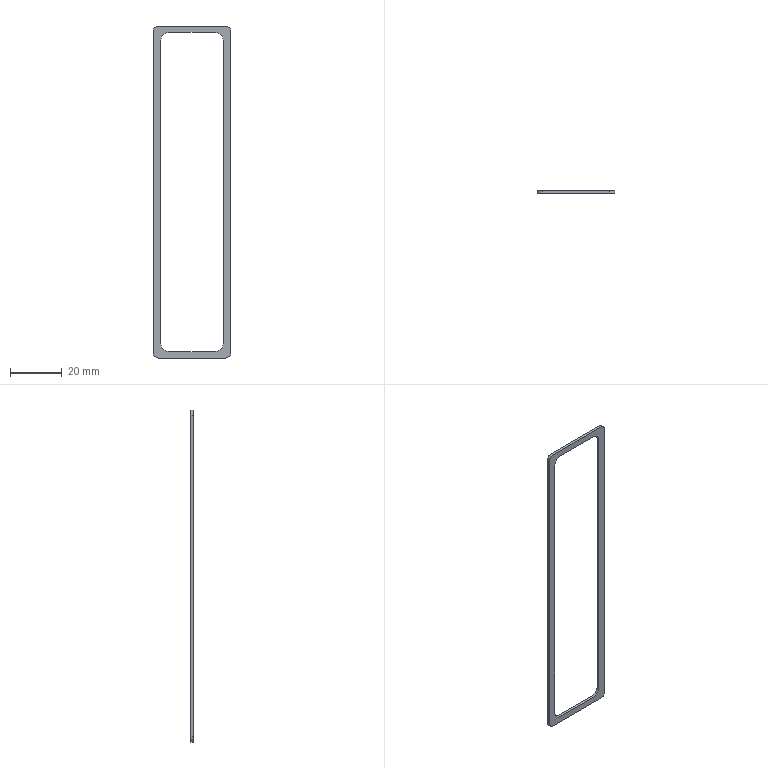Part | STEP file | _X2_751F4E45_X0_MS731-1_X2_8F_6 | 1 solid | 18 faces | box 30 x 1 x 128 mm | volume 892.292 mm3 | plane 10 | cylinder 8 | commonest cylinder face diameters 4 x4 6 x4
STEP:
#1=CARTESIAN_POINT('',(0.,0.,0.));
#2=DIRECTION('',(0.,0.,1.));
#3=DIRECTION('',(1.,0.,0.));
#4=AXIS2_PLACEMENT_3D('',#1,#2,#3);
#5=CARTESIAN_POINT('',(0.5,21.681,-127.));
#6=VERTEX_POINT('',#5);
#7=CARTESIAN_POINT('',(0.5,21.681,-3.));
#8=VERTEX_POINT('',#7);
#9=CARTESIAN_POINT('',(0.5,21.681,-127.));
#10=DIRECTION('',(0.,0.,1.));
#11=VECTOR('',#10,1.);
#12=LINE('',#9,#11);
#13=CARTESIAN_POINT('',(15.5,21.681,-65.));
#14=DIRECTION('',(0.,1.,0.));
#15=DIRECTION('',(-1.,0.,0.));
#16=AXIS2_PLACEMENT_3D('',#13,#14,#15);
#17=PLANE('',#16);
#18=CARTESIAN_POINT('',(15.,-62.));
#19=DIRECTION('',(0.,1.));
#20=VECTOR('',#19,1.);
#21=LINE('',#18,#20);
#22=(GEOMETRIC_REPRESENTATION_CONTEXT(2)PARAMETRIC_REPRESENTATION_CONTEXT()REPRESENTATION_CONTEXT('',''));
#23=DEFINITIONAL_REPRESENTATION('',(#21),#22);
#24=PCURVE('',#17,#23);
#25=CARTESIAN_POINT('',(0.5,21.681,-129.));
#26=DIRECTION('',(-1.,0.,0.));
#27=DIRECTION('',(0.,0.,-1.));
#28=AXIS2_PLACEMENT_3D('',#25,#26,#27);
#29=PLANE('',#28);
#30=CARTESIAN_POINT('',(-2.,0.));
#31=DIRECTION('',(-1.,0.));
#32=VECTOR('',#31,1.);
#33=LINE('',#30,#32);
#34=(GEOMETRIC_REPRESENTATION_CONTEXT(2)PARAMETRIC_REPRESENTATION_CONTEXT()REPRESENTATION_CONTEXT('',''));
#35=DEFINITIONAL_REPRESENTATION('',(#33),#34);
#36=PCURVE('',#29,#35);
#37=SURFACE_CURVE('',#12,(#24,#36),.PCURVE_S1.);
#38=EDGE_CURVE('',#6,#8,#37,.T.);
#39=ORIENTED_EDGE('',*,*,#38,.T.);
#40=CARTESIAN_POINT('',(2.5,21.681,-1.));
#41=VERTEX_POINT('',#40);
#42=CARTESIAN_POINT('',(2.5,21.681,-3.));
#43=DIRECTION('',(0.,-1.,0.));
#44=DIRECTION('',(0.,0.,1.));
#45=AXIS2_PLACEMENT_3D('',#42,#43,#44);
#46=CIRCLE('',#45,2.);
#47=CARTESIAN_POINT('',(13.,64.));
#48=CARTESIAN_POINT('',(16.464,64.));
#49=CARTESIAN_POINT('',(14.732,61.));
#50=CARTESIAN_POINT('',(13.,58.));
#51=CARTESIAN_POINT('',(11.268,61.));
#52=CARTESIAN_POINT('',(9.536,64.));
#53=CARTESIAN_POINT('',(13.,64.));
#54=(BOUNDED_CURVE()B_SPLINE_CURVE(2,(#47,#48,#49,#50,#51,#52,#53),.UNSPECIFIED.,.T.,.F.)B_SPLINE_CURVE_WITH_KNOTS((1,2,2,2,2,1),(-2.094,0.,2.094,4.189,6.283,8.378),.UNSPECIFIED.)CURVE()GEOMETRIC_REPRESENTATION_ITEM()RATIONAL_B_SPLINE_CURVE((1.,0.5,1.,0.5,1.,0.5,1.))REPRESENTATION_ITEM(''));
#55=(GEOMETRIC_REPRESENTATION_CONTEXT(2)PARAMETRIC_REPRESENTATION_CONTEXT()REPRESENTATION_CONTEXT('',''));
#56=DEFINITIONAL_REPRESENTATION('',(#54),#55);
#57=PCURVE('',#17,#56);
#58=CARTESIAN_POINT('',(2.5,22.908,-3.));
#59=DIRECTION('',(0.,-1.,0.));
#60=DIRECTION('',(0.,0.,-1.));
#61=AXIS2_PLACEMENT_3D('',#58,#59,#60);
#62=CYLINDRICAL_SURFACE('',#61,2.);
#63=CARTESIAN_POINT('',(3.142,1.226));
#64=DIRECTION('',(1.,0.));
#65=VECTOR('',#64,1.);
#66=LINE('',#63,#65);
#67=(GEOMETRIC_REPRESENTATION_CONTEXT(2)PARAMETRIC_REPRESENTATION_CONTEXT()REPRESENTATION_CONTEXT('',''));
#68=DEFINITIONAL_REPRESENTATION('',(#66),#67);
#69=PCURVE('',#62,#68);
#70=SURFACE_CURVE('',#46,(#57,#69),.PCURVE_S1.);
#71=EDGE_CURVE('',#41,#8,#70,.T.);
#72=ORIENTED_EDGE('',*,*,#71,.F.);
#73=CARTESIAN_POINT('',(28.5,21.681,-1.));
#74=VERTEX_POINT('',#73);
#75=CARTESIAN_POINT('',(2.5,21.681,-1.));
#76=DIRECTION('',(1.,0.,0.));
#77=VECTOR('',#76,1.);
#78=LINE('',#75,#77);
#79=CARTESIAN_POINT('',(13.,64.));
#80=DIRECTION('',(-1.,0.));
#81=VECTOR('',#80,1.);
#82=LINE('',#79,#81);
#83=(GEOMETRIC_REPRESENTATION_CONTEXT(2)PARAMETRIC_REPRESENTATION_CONTEXT()REPRESENTATION_CONTEXT('',''));
#84=DEFINITIONAL_REPRESENTATION('',(#82),#83);
#85=PCURVE('',#17,#84);
#86=CARTESIAN_POINT('',(0.5,21.681,-1.));
#87=DIRECTION('',(0.,0.,1.));
#88=DIRECTION('',(-1.,0.,0.));
#89=AXIS2_PLACEMENT_3D('',#86,#87,#88);
#90=PLANE('',#89);
#91=CARTESIAN_POINT('',(-2.,0.));
#92=DIRECTION('',(-1.,0.));
#93=VECTOR('',#92,1.);
#94=LINE('',#91,#93);
#95=(GEOMETRIC_REPRESENTATION_CONTEXT(2)PARAMETRIC_REPRESENTATION_CONTEXT()REPRESENTATION_CONTEXT('',''));
#96=DEFINITIONAL_REPRESENTATION('',(#94),#95);
#97=PCURVE('',#90,#96);
#98=SURFACE_CURVE('',#78,(#85,#97),.PCURVE_S1.);
#99=EDGE_CURVE('',#41,#74,#98,.T.);
#100=ORIENTED_EDGE('',*,*,#99,.T.);
#101=CARTESIAN_POINT('',(30.5,21.681,-3.));
#102=VERTEX_POINT('',#101);
#103=CARTESIAN_POINT('',(28.5,21.681,-3.));
#104=DIRECTION('',(0.,-1.,0.));
#105=DIRECTION('',(1.,0.,0.));
#106=AXIS2_PLACEMENT_3D('',#103,#104,#105);
#107=CIRCLE('',#106,2.);
#108=CARTESIAN_POINT('',(-15.,62.));
#109=CARTESIAN_POINT('',(-15.,65.464));
#110=CARTESIAN_POINT('',(-12.,63.732));
#111=CARTESIAN_POINT('',(-9.,62.));
#112=CARTESIAN_POINT('',(-12.,60.268));
#113=CARTESIAN_POINT('',(-15.,58.536));
#114=CARTESIAN_POINT('',(-15.,62.));
#115=(BOUNDED_CURVE()B_SPLINE_CURVE(2,(#108,#109,#110,#111,#112,#113,#114),.UNSPECIFIED.,.T.,.F.)B_SPLINE_CURVE_WITH_KNOTS((1,2,2,2,2,1),(-2.094,0.,2.094,4.189,6.283,8.378),.UNSPECIFIED.)CURVE()GEOMETRIC_REPRESENTATION_ITEM()RATIONAL_B_SPLINE_CURVE((1.,0.5,1.,0.5,1.,0.5,1.))REPRESENTATION_ITEM(''));
#116=(GEOMETRIC_REPRESENTATION_CONTEXT(2)PARAMETRIC_REPRESENTATION_CONTEXT()REPRESENTATION_CONTEXT('',''));
#117=DEFINITIONAL_REPRESENTATION('',(#115),#116);
#118=PCURVE('',#17,#117);
#119=CARTESIAN_POINT('',(28.5,22.908,-3.));
#120=DIRECTION('',(0.,-1.,0.));
#121=DIRECTION('',(-1.,0.,0.));
#122=AXIS2_PLACEMENT_3D('',#119,#120,#121);
#123=CYLINDRICAL_SURFACE('',#122,2.);
#124=CARTESIAN_POINT('',(3.142,1.226));
#125=DIRECTION('',(1.,0.));
#126=VECTOR('',#125,1.);
#127=LINE('',#124,#126);
#128=(GEOMETRIC_REPRESENTATION_CONTEXT(2)PARAMETRIC_REPRESENTATION_CONTEXT()REPRESENTATION_CONTEXT('',''));
#129=DEFINITIONAL_REPRESENTATION('',(#127),#128);
#130=PCURVE('',#123,#129);
#131=SURFACE_CURVE('',#107,(#118,#130),.PCURVE_S1.);
#132=EDGE_CURVE('',#102,#74,#131,.T.);
#133=ORIENTED_EDGE('',*,*,#132,.F.);
#134=CARTESIAN_POINT('',(30.5,21.681,-127.));
#135=VERTEX_POINT('',#134);
#136=CARTESIAN_POINT('',(30.5,21.681,-3.));
#137=DIRECTION('',(0.,0.,-1.));
#138=VECTOR('',#137,1.);
#139=LINE('',#136,#138);
#140=CARTESIAN_POINT('',(-15.,62.));
#141=DIRECTION('',(0.,-1.));
#142=VECTOR('',#141,1.);
#143=LINE('',#140,#142);
#144=(GEOMETRIC_REPRESENTATION_CONTEXT(2)PARAMETRIC_REPRESENTATION_CONTEXT()REPRESENTATION_CONTEXT('',''));
#145=DEFINITIONAL_REPRESENTATION('',(#143),#144);
#146=PCURVE('',#17,#145);
#147=CARTESIAN_POINT('',(30.5,21.681,-1.));
#148=DIRECTION('',(1.,0.,0.));
#149=DIRECTION('',(0.,0.,1.));
#150=AXIS2_PLACEMENT_3D('',#147,#148,#149);
#151=PLANE('',#150);
#152=CARTESIAN_POINT('',(-2.,0.));
#153=DIRECTION('',(-1.,0.));
#154=VECTOR('',#153,1.);
#155=LINE('',#152,#154);
#156=(GEOMETRIC_REPRESENTATION_CONTEXT(2)PARAMETRIC_REPRESENTATION_CONTEXT()REPRESENTATION_CONTEXT('',''));
#157=DEFINITIONAL_REPRESENTATION('',(#155),#156);
#158=PCURVE('',#151,#157);
#159=SURFACE_CURVE('',#139,(#146,#158),.PCURVE_S1.);
#160=EDGE_CURVE('',#102,#135,#159,.T.);
#161=ORIENTED_EDGE('',*,*,#160,.T.);
#162=CARTESIAN_POINT('',(28.5,21.681,-129.));
#163=VERTEX_POINT('',#162);
#164=CARTESIAN_POINT('',(28.5,21.681,-127.));
#165=DIRECTION('',(0.,-1.,0.));
#166=DIRECTION('',(0.,0.,-1.));
#167=AXIS2_PLACEMENT_3D('',#164,#165,#166);
#168=CIRCLE('',#167,2.);
#169=CARTESIAN_POINT('',(-13.,-64.));
#170=CARTESIAN_POINT('',(-16.464,-64.));
#171=CARTESIAN_POINT('',(-14.732,-61.));
#172=CARTESIAN_POINT('',(-13.,-58.));
#173=CARTESIAN_POINT('',(-11.268,-61.));
#174=CARTESIAN_POINT('',(-9.536,-64.));
#175=CARTESIAN_POINT('',(-13.,-64.));
#176=(BOUNDED_CURVE()B_SPLINE_CURVE(2,(#169,#170,#171,#172,#173,#174,#175),.UNSPECIFIED.,.T.,.F.)B_SPLINE_CURVE_WITH_KNOTS((1,2,2,2,2,1),(-2.094,0.,2.094,4.189,6.283,8.378),.UNSPECIFIED.)CURVE()GEOMETRIC_REPRESENTATION_ITEM()RATIONAL_B_SPLINE_CURVE((1.,0.5,1.,0.5,1.,0.5,1.))REPRESENTATION_ITEM(''));
#177=(GEOMETRIC_REPRESENTATION_CONTEXT(2)PARAMETRIC_REPRESENTATION_CONTEXT()REPRESENTATION_CONTEXT('',''));
#178=DEFINITIONAL_REPRESENTATION('',(#176),#177);
#179=PCURVE('',#17,#178);
#180=CARTESIAN_POINT('',(28.5,22.908,-127.));
#181=DIRECTION('',(0.,-1.,0.));
#182=DIRECTION('',(0.,0.,1.));
#183=AXIS2_PLACEMENT_3D('',#180,#181,#182);
#184=CYLINDRICAL_SURFACE('',#183,2.);
#185=CARTESIAN_POINT('',(3.142,1.226));
#186=DIRECTION('',(1.,0.));
#187=VECTOR('',#186,1.);
#188=LINE('',#185,#187);
#189=(GEOMETRIC_REPRESENTATION_CONTEXT(2)PARAMETRIC_REPRESENTATION_CONTEXT()REPRESENTATION_CONTEXT('',''));
#190=DEFINITIONAL_REPRESENTATION('',(#188),#189);
#191=PCURVE('',#184,#190);
#192=SURFACE_CURVE('',#168,(#179,#191),.PCURVE_S1.);
#193=EDGE_CURVE('',#163,#135,#192,.T.);
#194=ORIENTED_EDGE('',*,*,#193,.F.);
#195=CARTESIAN_POINT('',(2.5,21.681,-129.));
#196=VERTEX_POINT('',#195);
#197=CARTESIAN_POINT('',(28.5,21.681,-129.));
#198=DIRECTION('',(-1.,0.,0.));
#199=VECTOR('',#198,1.);
#200=LINE('',#197,#199);
#201=CARTESIAN_POINT('',(-13.,-64.));
#202=DIRECTION('',(1.,0.));
#203=VECTOR('',#202,1.);
#204=LINE('',#201,#203);
#205=(GEOMETRIC_REPRESENTATION_CONTEXT(2)PARAMETRIC_REPRESENTATION_CONTEXT()REPRESENTATION_CONTEXT('',''));
#206=DEFINITIONAL_REPRESENTATION('',(#204),#205);
#207=PCURVE('',#17,#206);
#208=CARTESIAN_POINT('',(30.5,21.681,-129.));
#209=DIRECTION('',(0.,0.,-1.));
#210=DIRECTION('',(1.,0.,0.));
#211=AXIS2_PLACEMENT_3D('',#208,#209,#210);
#212=PLANE('',#211);
#213=CARTESIAN_POINT('',(-2.,0.));
#214=DIRECTION('',(-1.,0.));
#215=VECTOR('',#214,1.);
#216=LINE('',#213,#215);
#217=(GEOMETRIC_REPRESENTATION_CONTEXT(2)PARAMETRIC_REPRESENTATION_CONTEXT()REPRESENTATION_CONTEXT('',''));
#218=DEFINITIONAL_REPRESENTATION('',(#216),#217);
#219=PCURVE('',#212,#218);
#220=SURFACE_CURVE('',#200,(#207,#219),.PCURVE_S1.);
#221=EDGE_CURVE('',#163,#196,#220,.T.);
#222=ORIENTED_EDGE('',*,*,#221,.T.);
#223=CARTESIAN_POINT('',(2.5,21.681,-127.));
#224=DIRECTION('',(0.,-1.,0.));
#225=DIRECTION('',(-1.,0.,0.));
#226=AXIS2_PLACEMENT_3D('',#223,#224,#225);
#227=CIRCLE('',#226,2.);
#228=CARTESIAN_POINT('',(15.,-62.));
#229=CARTESIAN_POINT('',(15.,-65.464));
#230=CARTESIAN_POINT('',(12.,-63.732));
#231=CARTESIAN_POINT('',(9.,-62.));
#232=CARTESIAN_POINT('',(12.,-60.268));
#233=CARTESIAN_POINT('',(15.,-58.536));
#234=CARTESIAN_POINT('',(15.,-62.));
#235=(BOUNDED_CURVE()B_SPLINE_CURVE(2,(#228,#229,#230,#231,#232,#233,#234),.UNSPECIFIED.,.T.,.F.)B_SPLINE_CURVE_WITH_KNOTS((1,2,2,2,2,1),(-2.094,0.,2.094,4.189,6.283,8.378),.UNSPECIFIED.)CURVE()GEOMETRIC_REPRESENTATION_ITEM()RATIONAL_B_SPLINE_CURVE((1.,0.5,1.,0.5,1.,0.5,1.))REPRESENTATION_ITEM(''));
#236=(GEOMETRIC_REPRESENTATION_CONTEXT(2)PARAMETRIC_REPRESENTATION_CONTEXT()REPRESENTATION_CONTEXT('',''));
#237=DEFINITIONAL_REPRESENTATION('',(#235),#236);
#238=PCURVE('',#17,#237);
#239=CARTESIAN_POINT('',(2.5,22.908,-127.));
#240=DIRECTION('',(0.,-1.,0.));
#241=DIRECTION('',(1.,0.,0.));
#242=AXIS2_PLACEMENT_3D('',#239,#240,#241);
#243=CYLINDRICAL_SURFACE('',#242,2.);
#244=CARTESIAN_POINT('',(3.142,1.226));
#245=DIRECTION('',(1.,0.));
#246=VECTOR('',#245,1.);
#247=LINE('',#244,#246);
#248=(GEOMETRIC_REPRESENTATION_CONTEXT(2)PARAMETRIC_REPRESENTATION_CONTEXT()REPRESENTATION_CONTEXT('',''));
#249=DEFINITIONAL_REPRESENTATION('',(#247),#248);
#250=PCURVE('',#243,#249);
#251=SURFACE_CURVE('',#227,(#238,#250),.PCURVE_S1.);
#252=EDGE_CURVE('',#6,#196,#251,.T.);
#253=ORIENTED_EDGE('',*,*,#252,.F.);
#254=EDGE_LOOP('',(#39,#72,#100,#133,#161,#194,#222,#253));
#255=FACE_BOUND('',#254,.F.);
#256=CARTESIAN_POINT('',(6.5,21.681,-126.5));
#257=VERTEX_POINT('',#256);
#258=CARTESIAN_POINT('',(3.5,21.681,-123.5));
#259=VERTEX_POINT('',#258);
#260=CARTESIAN_POINT('',(6.5,21.681,-123.5));
#261=DIRECTION('',(0.,1.,0.));
#262=DIRECTION('',(0.,0.,-1.));
#263=AXIS2_PLACEMENT_3D('',#260,#261,#262);
#264=CIRCLE('',#263,3.);
#265=CARTESIAN_POINT('',(9.,-58.5));
#266=DIRECTION('',(0.,-1.));
#267=AXIS2_PLACEMENT_2D('',#265,#266);
#268=CIRCLE('',#267,3.);
#269=(GEOMETRIC_REPRESENTATION_CONTEXT(2)PARAMETRIC_REPRESENTATION_CONTEXT()REPRESENTATION_CONTEXT('',''));
#270=DEFINITIONAL_REPRESENTATION('',(#268),#269);
#271=PCURVE('',#17,#270);
#272=CARTESIAN_POINT('',(6.5,21.488,-123.5));
#273=DIRECTION('',(0.,1.,0.));
#274=DIRECTION('',(0.,0.,1.));
#275=AXIS2_PLACEMENT_3D('',#272,#273,#274);
#276=CYLINDRICAL_SURFACE('',#275,3.);
#277=CARTESIAN_POINT('',(3.142,0.1933));
#278=DIRECTION('',(1.,0.));
#279=VECTOR('',#278,1.);
#280=LINE('',#277,#279);
#281=(GEOMETRIC_REPRESENTATION_CONTEXT(2)PARAMETRIC_REPRESENTATION_CONTEXT()REPRESENTATION_CONTEXT('',''));
#282=DEFINITIONAL_REPRESENTATION('',(#280),#281);
#283=PCURVE('',#276,#282);
#284=SURFACE_CURVE('',#264,(#271,#283),.PCURVE_S1.);
#285=EDGE_CURVE('',#257,#259,#284,.T.);
#286=ORIENTED_EDGE('',*,*,#285,.F.);
#287=CARTESIAN_POINT('',(24.5,21.681,-126.5));
#288=VERTEX_POINT('',#287);
#289=CARTESIAN_POINT('',(6.5,21.681,-126.5));
#290=DIRECTION('',(1.,0.,0.));
#291=VECTOR('',#290,1.);
#292=LINE('',#289,#291);
#293=CARTESIAN_POINT('',(9.,-61.5));
#294=DIRECTION('',(-1.,0.));
#295=VECTOR('',#294,1.);
#296=LINE('',#293,#295);
#297=(GEOMETRIC_REPRESENTATION_CONTEXT(2)PARAMETRIC_REPRESENTATION_CONTEXT()REPRESENTATION_CONTEXT('',''));
#298=DEFINITIONAL_REPRESENTATION('',(#296),#297);
#299=PCURVE('',#17,#298);
#300=CARTESIAN_POINT('',(3.5,21.681,-126.5));
#301=DIRECTION('',(0.,0.,1.));
#302=DIRECTION('',(-1.,0.,0.));
#303=AXIS2_PLACEMENT_3D('',#300,#301,#302);
#304=PLANE('',#303);
#305=CARTESIAN_POINT('',(-3.,0.));
#306=DIRECTION('',(-1.,0.));
#307=VECTOR('',#306,1.);
#308=LINE('',#305,#307);
#309=(GEOMETRIC_REPRESENTATION_CONTEXT(2)PARAMETRIC_REPRESENTATION_CONTEXT()REPRESENTATION_CONTEXT('',''));
#310=DEFINITIONAL_REPRESENTATION('',(#308),#309);
#311=PCURVE('',#304,#310);
#312=SURFACE_CURVE('',#292,(#299,#311),.PCURVE_S1.);
#313=EDGE_CURVE('',#257,#288,#312,.T.);
#314=ORIENTED_EDGE('',*,*,#313,.T.);
#315=CARTESIAN_POINT('',(27.5,21.681,-123.5));
#316=VERTEX_POINT('',#315);
#317=CARTESIAN_POINT('',(24.5,21.681,-123.5));
#318=DIRECTION('',(0.,1.,0.));
#319=DIRECTION('',(1.,0.,0.));
#320=AXIS2_PLACEMENT_3D('',#317,#318,#319);
#321=CIRCLE('',#320,3.);
#322=CARTESIAN_POINT('',(-9.,-58.5));
#323=DIRECTION('',(-1.,0.));
#324=AXIS2_PLACEMENT_2D('',#322,#323);
#325=CIRCLE('',#324,3.);
#326=(GEOMETRIC_REPRESENTATION_CONTEXT(2)PARAMETRIC_REPRESENTATION_CONTEXT()REPRESENTATION_CONTEXT('',''));
#327=DEFINITIONAL_REPRESENTATION('',(#325),#326);
#328=PCURVE('',#17,#327);
#329=CARTESIAN_POINT('',(24.5,21.488,-123.5));
#330=DIRECTION('',(0.,1.,0.));
#331=DIRECTION('',(-1.,0.,0.));
#332=AXIS2_PLACEMENT_3D('',#329,#330,#331);
#333=CYLINDRICAL_SURFACE('',#332,3.);
#334=CARTESIAN_POINT('',(3.142,0.1933));
#335=DIRECTION('',(1.,0.));
#336=VECTOR('',#335,1.);
#337=LINE('',#334,#336);
#338=(GEOMETRIC_REPRESENTATION_CONTEXT(2)PARAMETRIC_REPRESENTATION_CONTEXT()REPRESENTATION_CONTEXT('',''));
#339=DEFINITIONAL_REPRESENTATION('',(#337),#338);
#340=PCURVE('',#333,#339);
#341=SURFACE_CURVE('',#321,(#328,#340),.PCURVE_S1.);
#342=EDGE_CURVE('',#316,#288,#341,.T.);
#343=ORIENTED_EDGE('',*,*,#342,.F.);
#344=CARTESIAN_POINT('',(27.5,21.681,-6.5));
#345=VERTEX_POINT('',#344);
#346=CARTESIAN_POINT('',(27.5,21.681,-123.5));
#347=DIRECTION('',(0.,0.,1.));
#348=VECTOR('',#347,1.);
#349=LINE('',#346,#348);
#350=CARTESIAN_POINT('',(-12.,-58.5));
#351=DIRECTION('',(0.,1.));
#352=VECTOR('',#351,1.);
#353=LINE('',#350,#352);
#354=(GEOMETRIC_REPRESENTATION_CONTEXT(2)PARAMETRIC_REPRESENTATION_CONTEXT()REPRESENTATION_CONTEXT('',''));
#355=DEFINITIONAL_REPRESENTATION('',(#353),#354);
#356=PCURVE('',#17,#355);
#357=CARTESIAN_POINT('',(27.5,21.681,-126.5));
#358=DIRECTION('',(-1.,0.,0.));
#359=DIRECTION('',(0.,0.,-1.));
#360=AXIS2_PLACEMENT_3D('',#357,#358,#359);
#361=PLANE('',#360);
#362=CARTESIAN_POINT('',(-3.,0.));
#363=DIRECTION('',(-1.,0.));
#364=VECTOR('',#363,1.);
#365=LINE('',#362,#364);
#366=(GEOMETRIC_REPRESENTATION_CONTEXT(2)PARAMETRIC_REPRESENTATION_CONTEXT()REPRESENTATION_CONTEXT('',''));
#367=DEFINITIONAL_REPRESENTATION('',(#365),#366);
#368=PCURVE('',#361,#367);
#369=SURFACE_CURVE('',#349,(#356,#368),.PCURVE_S1.);
#370=EDGE_CURVE('',#316,#345,#369,.T.);
#371=ORIENTED_EDGE('',*,*,#370,.T.);
#372=CARTESIAN_POINT('',(24.5,21.681,-3.5));
#373=VERTEX_POINT('',#372);
#374=CARTESIAN_POINT('',(24.5,21.681,-6.5));
#375=DIRECTION('',(0.,1.,0.));
#376=DIRECTION('',(0.,0.,1.));
#377=AXIS2_PLACEMENT_3D('',#374,#375,#376);
#378=CIRCLE('',#377,3.);
#379=CARTESIAN_POINT('',(-9.,58.5));
#380=DIRECTION('',(0.,1.));
#381=AXIS2_PLACEMENT_2D('',#379,#380);
#382=CIRCLE('',#381,3.);
#383=(GEOMETRIC_REPRESENTATION_CONTEXT(2)PARAMETRIC_REPRESENTATION_CONTEXT()REPRESENTATION_CONTEXT('',''));
#384=DEFINITIONAL_REPRESENTATION('',(#382),#383);
#385=PCURVE('',#17,#384);
#386=CARTESIAN_POINT('',(24.5,21.488,-6.5));
#387=DIRECTION('',(0.,1.,0.));
#388=DIRECTION('',(0.,0.,-1.));
#389=AXIS2_PLACEMENT_3D('',#386,#387,#388);
#390=CYLINDRICAL_SURFACE('',#389,3.);
#391=CARTESIAN_POINT('',(3.142,0.1933));
#392=DIRECTION('',(1.,0.));
#393=VECTOR('',#392,1.);
#394=LINE('',#391,#393);
#395=(GEOMETRIC_REPRESENTATION_CONTEXT(2)PARAMETRIC_REPRESENTATION_CONTEXT()REPRESENTATION_CONTEXT('',''));
#396=DEFINITIONAL_REPRESENTATION('',(#394),#395);
#397=PCURVE('',#390,#396);
#398=SURFACE_CURVE('',#378,(#385,#397),.PCURVE_S1.);
#399=EDGE_CURVE('',#373,#345,#398,.T.);
#400=ORIENTED_EDGE('',*,*,#399,.F.);
#401=CARTESIAN_POINT('',(6.5,21.681,-3.5));
#402=VERTEX_POINT('',#401);
#403=CARTESIAN_POINT('',(24.5,21.681,-3.5));
#404=DIRECTION('',(-1.,0.,0.));
#405=VECTOR('',#404,1.);
#406=LINE('',#403,#405);
#407=CARTESIAN_POINT('',(-9.,61.5));
#408=DIRECTION('',(1.,0.));
#409=VECTOR('',#408,1.);
#410=LINE('',#407,#409);
#411=(GEOMETRIC_REPRESENTATION_CONTEXT(2)PARAMETRIC_REPRESENTATION_CONTEXT()REPRESENTATION_CONTEXT('',''));
#412=DEFINITIONAL_REPRESENTATION('',(#410),#411);
#413=PCURVE('',#17,#412);
#414=CARTESIAN_POINT('',(27.5,21.681,-3.5));
#415=DIRECTION('',(0.,0.,-1.));
#416=DIRECTION('',(1.,0.,0.));
#417=AXIS2_PLACEMENT_3D('',#414,#415,#416);
#418=PLANE('',#417);
#419=CARTESIAN_POINT('',(-3.,0.));
#420=DIRECTION('',(-1.,0.));
#421=VECTOR('',#420,1.);
#422=LINE('',#419,#421);
#423=(GEOMETRIC_REPRESENTATION_CONTEXT(2)PARAMETRIC_REPRESENTATION_CONTEXT()REPRESENTATION_CONTEXT('',''));
#424=DEFINITIONAL_REPRESENTATION('',(#422),#423);
#425=PCURVE('',#418,#424);
#426=SURFACE_CURVE('',#406,(#413,#425),.PCURVE_S1.);
#427=EDGE_CURVE('',#373,#402,#426,.T.);
#428=ORIENTED_EDGE('',*,*,#427,.T.);
#429=CARTESIAN_POINT('',(3.5,21.681,-6.5));
#430=VERTEX_POINT('',#429);
#431=CARTESIAN_POINT('',(6.5,21.681,-6.5));
#432=DIRECTION('',(0.,1.,0.));
#433=DIRECTION('',(-1.,0.,0.));
#434=AXIS2_PLACEMENT_3D('',#431,#432,#433);
#435=CIRCLE('',#434,3.);
#436=CARTESIAN_POINT('',(9.,58.5));
#437=DIRECTION('',(1.,0.));
#438=AXIS2_PLACEMENT_2D('',#436,#437);
#439=CIRCLE('',#438,3.);
#440=(GEOMETRIC_REPRESENTATION_CONTEXT(2)PARAMETRIC_REPRESENTATION_CONTEXT()REPRESENTATION_CONTEXT('',''));
#441=DEFINITIONAL_REPRESENTATION('',(#439),#440);
#442=PCURVE('',#17,#441);
#443=CARTESIAN_POINT('',(6.5,21.488,-6.5));
#444=DIRECTION('',(0.,1.,0.));
#445=DIRECTION('',(1.,0.,0.));
#446=AXIS2_PLACEMENT_3D('',#443,#444,#445);
#447=CYLINDRICAL_SURFACE('',#446,3.);
#448=CARTESIAN_POINT('',(3.142,0.1933));
#449=DIRECTION('',(1.,0.));
#450=VECTOR('',#449,1.);
#451=LINE('',#448,#450);
#452=(GEOMETRIC_REPRESENTATION_CONTEXT(2)PARAMETRIC_REPRESENTATION_CONTEXT()REPRESENTATION_CONTEXT('',''));
#453=DEFINITIONAL_REPRESENTATION('',(#451),#452);
#454=PCURVE('',#447,#453);
#455=SURFACE_CURVE('',#435,(#442,#454),.PCURVE_S1.);
#456=EDGE_CURVE('',#430,#402,#455,.T.);
#457=ORIENTED_EDGE('',*,*,#456,.F.);
#458=CARTESIAN_POINT('',(3.5,21.681,-6.5));
#459=DIRECTION('',(0.,0.,-1.));
#460=VECTOR('',#459,1.);
#461=LINE('',#458,#460);
#462=CARTESIAN_POINT('',(12.,58.5));
#463=DIRECTION('',(0.,-1.));
#464=VECTOR('',#463,1.);
#465=LINE('',#462,#464);
#466=(GEOMETRIC_REPRESENTATION_CONTEXT(2)PARAMETRIC_REPRESENTATION_CONTEXT()REPRESENTATION_CONTEXT('',''));
#467=DEFINITIONAL_REPRESENTATION('',(#465),#466);
#468=PCURVE('',#17,#467);
#469=CARTESIAN_POINT('',(3.5,21.681,-3.5));
#470=DIRECTION('',(1.,0.,0.));
#471=DIRECTION('',(0.,0.,1.));
#472=AXIS2_PLACEMENT_3D('',#469,#470,#471);
#473=PLANE('',#472);
#474=CARTESIAN_POINT('',(-3.,0.));
#475=DIRECTION('',(-1.,0.));
#476=VECTOR('',#475,1.);
#477=LINE('',#474,#476);
#478=(GEOMETRIC_REPRESENTATION_CONTEXT(2)PARAMETRIC_REPRESENTATION_CONTEXT()REPRESENTATION_CONTEXT('',''));
#479=DEFINITIONAL_REPRESENTATION('',(#477),#478);
#480=PCURVE('',#473,#479);
#481=SURFACE_CURVE('',#461,(#468,#480),.PCURVE_S1.);
#482=EDGE_CURVE('',#430,#259,#481,.T.);
#483=ORIENTED_EDGE('',*,*,#482,.T.);
#484=EDGE_LOOP('',(#286,#314,#343,#371,#400,#428,#457,#483));
#485=FACE_BOUND('',#484,.F.);
#486=ADVANCED_FACE('',(#255,#485),#17,.F.);
#487=CARTESIAN_POINT('',(0.5,22.681,-127.));
#488=VERTEX_POINT('',#487);
#489=CARTESIAN_POINT('',(0.5,22.681,-3.));
#490=VERTEX_POINT('',#489);
#491=CARTESIAN_POINT('',(0.5,22.681,-127.));
#492=DIRECTION('',(0.,0.,1.));
#493=VECTOR('',#492,1.);
#494=LINE('',#491,#493);
#495=CARTESIAN_POINT('',(-2.,-1.));
#496=DIRECTION('',(-1.,0.));
#497=VECTOR('',#496,1.);
#498=LINE('',#495,#497);
#499=(GEOMETRIC_REPRESENTATION_CONTEXT(2)PARAMETRIC_REPRESENTATION_CONTEXT()REPRESENTATION_CONTEXT('',''));
#500=DEFINITIONAL_REPRESENTATION('',(#498),#499);
#501=PCURVE('',#29,#500);
#502=CARTESIAN_POINT('',(15.5,22.681,-65.));
#503=DIRECTION('',(0.,1.,0.));
#504=DIRECTION('',(-1.,0.,0.));
#505=AXIS2_PLACEMENT_3D('',#502,#503,#504);
#506=PLANE('',#505);
#507=CARTESIAN_POINT('',(15.,-62.));
#508=DIRECTION('',(0.,1.));
#509=VECTOR('',#508,1.);
#510=LINE('',#507,#509);
#511=(GEOMETRIC_REPRESENTATION_CONTEXT(2)PARAMETRIC_REPRESENTATION_CONTEXT()REPRESENTATION_CONTEXT('',''));
#512=DEFINITIONAL_REPRESENTATION('',(#510),#511);
#513=PCURVE('',#506,#512);
#514=SURFACE_CURVE('',#494,(#501,#513),.PCURVE_S1.);
#515=EDGE_CURVE('',#488,#490,#514,.T.);
#516=ORIENTED_EDGE('',*,*,#515,.T.);
#517=CARTESIAN_POINT('',(0.5,22.681,-3.));
#518=DIRECTION('',(0.,-1.,0.));
#519=VECTOR('',#518,1.);
#520=LINE('',#517,#519);
#521=CARTESIAN_POINT('',(-126.,-1.));
#522=DIRECTION('',(0.,1.));
#523=VECTOR('',#522,1.);
#524=LINE('',#521,#523);
#525=(GEOMETRIC_REPRESENTATION_CONTEXT(2)PARAMETRIC_REPRESENTATION_CONTEXT()REPRESENTATION_CONTEXT('',''));
#526=DEFINITIONAL_REPRESENTATION('',(#524),#525);
#527=PCURVE('',#29,#526);
#528=CARTESIAN_POINT('',(4.712,0.2263));
#529=DIRECTION('',(0.,1.));
#530=VECTOR('',#529,1.);
#531=LINE('',#528,#530);
#532=(GEOMETRIC_REPRESENTATION_CONTEXT(2)PARAMETRIC_REPRESENTATION_CONTEXT()REPRESENTATION_CONTEXT('',''));
#533=DEFINITIONAL_REPRESENTATION('',(#531),#532);
#534=PCURVE('',#62,#533);
#535=SURFACE_CURVE('',#520,(#527,#534),.PCURVE_S1.);
#536=EDGE_CURVE('',#490,#8,#535,.T.);
#537=ORIENTED_EDGE('',*,*,#536,.T.);
#538=ORIENTED_EDGE('',*,*,#38,.F.);
#539=CARTESIAN_POINT('',(0.5,21.681,-127.));
#540=DIRECTION('',(0.,1.,0.));
#541=VECTOR('',#540,1.);
#542=LINE('',#539,#541);
#543=CARTESIAN_POINT('',(-2.,0.));
#544=DIRECTION('',(0.,-1.));
#545=VECTOR('',#544,1.);
#546=LINE('',#543,#545);
#547=(GEOMETRIC_REPRESENTATION_CONTEXT(2)PARAMETRIC_REPRESENTATION_CONTEXT()REPRESENTATION_CONTEXT('',''));
#548=DEFINITIONAL_REPRESENTATION('',(#546),#547);
#549=PCURVE('',#29,#548);
#550=CARTESIAN_POINT('',(3.142,1.226));
#551=DIRECTION('',(0.,-1.));
#552=VECTOR('',#551,1.);
#553=LINE('',#550,#552);
#554=(GEOMETRIC_REPRESENTATION_CONTEXT(2)PARAMETRIC_REPRESENTATION_CONTEXT()REPRESENTATION_CONTEXT('',''));
#555=DEFINITIONAL_REPRESENTATION('',(#553),#554);
#556=PCURVE('',#243,#555);
#557=SURFACE_CURVE('',#542,(#549,#556),.PCURVE_S1.);
#558=EDGE_CURVE('',#6,#488,#557,.T.);
#559=ORIENTED_EDGE('',*,*,#558,.T.);
#560=EDGE_LOOP('',(#516,#537,#538,#559));
#561=FACE_BOUND('',#560,.F.);
#562=ADVANCED_FACE('',(#561),#29,.T.);
#563=CARTESIAN_POINT('',(2.5,22.681,-1.));
#564=VERTEX_POINT('',#563);
#565=CARTESIAN_POINT('',(28.5,22.681,-1.));
#566=VERTEX_POINT('',#565);
#567=CARTESIAN_POINT('',(2.5,22.681,-1.));
#568=DIRECTION('',(1.,0.,0.));
#569=VECTOR('',#568,1.);
#570=LINE('',#567,#569);
#571=CARTESIAN_POINT('',(13.,64.));
#572=DIRECTION('',(-1.,0.));
#573=VECTOR('',#572,1.);
#574=LINE('',#571,#573);
#575=(GEOMETRIC_REPRESENTATION_CONTEXT(2)PARAMETRIC_REPRESENTATION_CONTEXT()REPRESENTATION_CONTEXT('',''));
#576=DEFINITIONAL_REPRESENTATION('',(#574),#575);
#577=PCURVE('',#506,#576);
#578=CARTESIAN_POINT('',(-2.,-1.));
#579=DIRECTION('',(-1.,0.));
#580=VECTOR('',#579,1.);
#581=LINE('',#578,#580);
#582=(GEOMETRIC_REPRESENTATION_CONTEXT(2)PARAMETRIC_REPRESENTATION_CONTEXT()REPRESENTATION_CONTEXT('',''));
#583=DEFINITIONAL_REPRESENTATION('',(#581),#582);
#584=PCURVE('',#90,#583);
#585=SURFACE_CURVE('',#570,(#577,#584),.PCURVE_S1.);
#586=EDGE_CURVE('',#564,#566,#585,.T.);
#587=ORIENTED_EDGE('',*,*,#586,.F.);
#588=CARTESIAN_POINT('',(2.5,22.681,-3.));
#589=DIRECTION('',(0.,1.,0.));
#590=DIRECTION('',(-1.,0.,0.));
#591=AXIS2_PLACEMENT_3D('',#588,#589,#590);
#592=CIRCLE('',#591,2.);
#593=CARTESIAN_POINT('',(13.,62.));
#594=DIRECTION('',(1.,0.));
#595=AXIS2_PLACEMENT_2D('',#593,#594);
#596=CIRCLE('',#595,2.);
#597=(GEOMETRIC_REPRESENTATION_CONTEXT(2)PARAMETRIC_REPRESENTATION_CONTEXT()REPRESENTATION_CONTEXT('',''));
#598=DEFINITIONAL_REPRESENTATION('',(#596),#597);
#599=PCURVE('',#506,#598);
#600=CARTESIAN_POINT('',(4.712,0.2263));
#601=DIRECTION('',(-1.,0.));
#602=VECTOR('',#601,1.);
#603=LINE('',#600,#602);
#604=(GEOMETRIC_REPRESENTATION_CONTEXT(2)PARAMETRIC_REPRESENTATION_CONTEXT()REPRESENTATION_CONTEXT('',''));
#605=DEFINITIONAL_REPRESENTATION('',(#603),#604);
#606=PCURVE('',#62,#605);
#607=SURFACE_CURVE('',#592,(#599,#606),.PCURVE_S1.);
#608=EDGE_CURVE('',#490,#564,#607,.T.);
#609=ORIENTED_EDGE('',*,*,#608,.F.);
#610=ORIENTED_EDGE('',*,*,#515,.F.);
#611=CARTESIAN_POINT('',(2.5,22.681,-129.));
#612=VERTEX_POINT('',#611);
#613=CARTESIAN_POINT('',(2.5,22.681,-127.));
#614=DIRECTION('',(0.,1.,0.));
#615=DIRECTION('',(0.,0.,-1.));
#616=AXIS2_PLACEMENT_3D('',#613,#614,#615);
#617=CIRCLE('',#616,2.);
#618=CARTESIAN_POINT('',(13.,-62.));
#619=DIRECTION('',(0.,-1.));
#620=AXIS2_PLACEMENT_2D('',#618,#619);
#621=CIRCLE('',#620,2.);
#622=(GEOMETRIC_REPRESENTATION_CONTEXT(2)PARAMETRIC_REPRESENTATION_CONTEXT()REPRESENTATION_CONTEXT('',''));
#623=DEFINITIONAL_REPRESENTATION('',(#621),#622);
#624=PCURVE('',#506,#623);
#625=CARTESIAN_POINT('',(4.712,0.2263));
#626=DIRECTION('',(-1.,0.));
#627=VECTOR('',#626,1.);
#628=LINE('',#625,#627);
#629=(GEOMETRIC_REPRESENTATION_CONTEXT(2)PARAMETRIC_REPRESENTATION_CONTEXT()REPRESENTATION_CONTEXT('',''));
#630=DEFINITIONAL_REPRESENTATION('',(#628),#629);
#631=PCURVE('',#243,#630);
#632=SURFACE_CURVE('',#617,(#624,#631),.PCURVE_S1.);
#633=EDGE_CURVE('',#612,#488,#632,.T.);
#634=ORIENTED_EDGE('',*,*,#633,.F.);
#635=CARTESIAN_POINT('',(28.5,22.681,-129.));
#636=VERTEX_POINT('',#635);
#637=CARTESIAN_POINT('',(28.5,22.681,-129.));
#638=DIRECTION('',(-1.,0.,0.));
#639=VECTOR('',#638,1.);
#640=LINE('',#637,#639);
#641=CARTESIAN_POINT('',(-13.,-64.));
#642=DIRECTION('',(1.,0.));
#643=VECTOR('',#642,1.);
#644=LINE('',#641,#643);
#645=(GEOMETRIC_REPRESENTATION_CONTEXT(2)PARAMETRIC_REPRESENTATION_CONTEXT()REPRESENTATION_CONTEXT('',''));
#646=DEFINITIONAL_REPRESENTATION('',(#644),#645);
#647=PCURVE('',#506,#646);
#648=CARTESIAN_POINT('',(-2.,-1.));
#649=DIRECTION('',(-1.,0.));
#650=VECTOR('',#649,1.);
#651=LINE('',#648,#650);
#652=(GEOMETRIC_REPRESENTATION_CONTEXT(2)PARAMETRIC_REPRESENTATION_CONTEXT()REPRESENTATION_CONTEXT('',''));
#653=DEFINITIONAL_REPRESENTATION('',(#651),#652);
#654=PCURVE('',#212,#653);
#655=SURFACE_CURVE('',#640,(#647,#654),.PCURVE_S1.);
#656=EDGE_CURVE('',#636,#612,#655,.T.);
#657=ORIENTED_EDGE('',*,*,#656,.F.);
#658=CARTESIAN_POINT('',(30.5,22.681,-127.));
#659=VERTEX_POINT('',#658);
#660=CARTESIAN_POINT('',(28.5,22.681,-127.));
#661=DIRECTION('',(0.,1.,0.));
#662=DIRECTION('',(1.,0.,0.));
#663=AXIS2_PLACEMENT_3D('',#660,#661,#662);
#664=CIRCLE('',#663,2.);
#665=CARTESIAN_POINT('',(-13.,-62.));
#666=DIRECTION('',(-1.,0.));
#667=AXIS2_PLACEMENT_2D('',#665,#666);
#668=CIRCLE('',#667,2.);
#669=(GEOMETRIC_REPRESENTATION_CONTEXT(2)PARAMETRIC_REPRESENTATION_CONTEXT()REPRESENTATION_CONTEXT('',''));
#670=DEFINITIONAL_REPRESENTATION('',(#668),#669);
#671=PCURVE('',#506,#670);
#672=CARTESIAN_POINT('',(4.712,0.2263));
#673=DIRECTION('',(-1.,0.));
#674=VECTOR('',#673,1.);
#675=LINE('',#672,#674);
#676=(GEOMETRIC_REPRESENTATION_CONTEXT(2)PARAMETRIC_REPRESENTATION_CONTEXT()REPRESENTATION_CONTEXT('',''));
#677=DEFINITIONAL_REPRESENTATION('',(#675),#676);
#678=PCURVE('',#184,#677);
#679=SURFACE_CURVE('',#664,(#671,#678),.PCURVE_S1.);
#680=EDGE_CURVE('',#659,#636,#679,.T.);
#681=ORIENTED_EDGE('',*,*,#680,.F.);
#682=CARTESIAN_POINT('',(30.5,22.681,-3.));
#683=VERTEX_POINT('',#682);
#684=CARTESIAN_POINT('',(30.5,22.681,-3.));
#685=DIRECTION('',(0.,0.,-1.));
#686=VECTOR('',#685,1.);
#687=LINE('',#684,#686);
#688=CARTESIAN_POINT('',(-15.,62.));
#689=DIRECTION('',(0.,-1.));
#690=VECTOR('',#689,1.);
#691=LINE('',#688,#690);
#692=(GEOMETRIC_REPRESENTATION_CONTEXT(2)PARAMETRIC_REPRESENTATION_CONTEXT()REPRESENTATION_CONTEXT('',''));
#693=DEFINITIONAL_REPRESENTATION('',(#691),#692);
#694=PCURVE('',#506,#693);
#695=CARTESIAN_POINT('',(-2.,-1.));
#696=DIRECTION('',(-1.,0.));
#697=VECTOR('',#696,1.);
#698=LINE('',#695,#697);
#699=(GEOMETRIC_REPRESENTATION_CONTEXT(2)PARAMETRIC_REPRESENTATION_CONTEXT()REPRESENTATION_CONTEXT('',''));
#700=DEFINITIONAL_REPRESENTATION('',(#698),#699);
#701=PCURVE('',#151,#700);
#702=SURFACE_CURVE('',#687,(#694,#701),.PCURVE_S1.);
#703=EDGE_CURVE('',#683,#659,#702,.T.);
#704=ORIENTED_EDGE('',*,*,#703,.F.);
#705=CARTESIAN_POINT('',(28.5,22.681,-3.));
#706=DIRECTION('',(0.,1.,0.));
#707=DIRECTION('',(0.,0.,1.));
#708=AXIS2_PLACEMENT_3D('',#705,#706,#707);
#709=CIRCLE('',#708,2.);
#710=CARTESIAN_POINT('',(-13.,62.));
#711=DIRECTION('',(0.,1.));
#712=AXIS2_PLACEMENT_2D('',#710,#711);
#713=CIRCLE('',#712,2.);
#714=(GEOMETRIC_REPRESENTATION_CONTEXT(2)PARAMETRIC_REPRESENTATION_CONTEXT()REPRESENTATION_CONTEXT('',''));
#715=DEFINITIONAL_REPRESENTATION('',(#713),#714);
#716=PCURVE('',#506,#715);
#717=CARTESIAN_POINT('',(4.712,0.2263));
#718=DIRECTION('',(-1.,0.));
#719=VECTOR('',#718,1.);
#720=LINE('',#717,#719);
#721=(GEOMETRIC_REPRESENTATION_CONTEXT(2)PARAMETRIC_REPRESENTATION_CONTEXT()REPRESENTATION_CONTEXT('',''));
#722=DEFINITIONAL_REPRESENTATION('',(#720),#721);
#723=PCURVE('',#123,#722);
#724=SURFACE_CURVE('',#709,(#716,#723),.PCURVE_S1.);
#725=EDGE_CURVE('',#566,#683,#724,.T.);
#726=ORIENTED_EDGE('',*,*,#725,.F.);
#727=EDGE_LOOP('',(#587,#609,#610,#634,#657,#681,#704,#726));
#728=FACE_BOUND('',#727,.F.);
#729=CARTESIAN_POINT('',(27.5,22.681,-6.5));
#730=VERTEX_POINT('',#729);
#731=CARTESIAN_POINT('',(24.5,22.681,-3.5));
#732=VERTEX_POINT('',#731);
#733=CARTESIAN_POINT('',(24.5,22.681,-6.5));
#734=DIRECTION('',(0.,-1.,0.));
#735=DIRECTION('',(1.,0.,0.));
#736=AXIS2_PLACEMENT_3D('',#733,#734,#735);
#737=CIRCLE('',#736,3.);
#738=CARTESIAN_POINT('',(-12.,58.5));
#739=CARTESIAN_POINT('',(-12.,63.696));
#740=CARTESIAN_POINT('',(-7.5,61.098));
#741=CARTESIAN_POINT('',(-3.,58.5));
#742=CARTESIAN_POINT('',(-7.5,55.902));
#743=CARTESIAN_POINT('',(-12.,53.304));
#744=CARTESIAN_POINT('',(-12.,58.5));
#745=(BOUNDED_CURVE()B_SPLINE_CURVE(2,(#738,#739,#740,#741,#742,#743,#744),.UNSPECIFIED.,.T.,.F.)B_SPLINE_CURVE_WITH_KNOTS((1,2,2,2,2,1),(-2.094,0.,2.094,4.189,6.283,8.378),.UNSPECIFIED.)CURVE()GEOMETRIC_REPRESENTATION_ITEM()RATIONAL_B_SPLINE_CURVE((1.,0.5,1.,0.5,1.,0.5,1.))REPRESENTATION_ITEM(''));
#746=(GEOMETRIC_REPRESENTATION_CONTEXT(2)PARAMETRIC_REPRESENTATION_CONTEXT()REPRESENTATION_CONTEXT('',''));
#747=DEFINITIONAL_REPRESENTATION('',(#745),#746);
#748=PCURVE('',#506,#747);
#749=CARTESIAN_POINT('',(4.712,1.193));
#750=DIRECTION('',(-1.,0.));
#751=VECTOR('',#750,1.);
#752=LINE('',#749,#751);
#753=(GEOMETRIC_REPRESENTATION_CONTEXT(2)PARAMETRIC_REPRESENTATION_CONTEXT()REPRESENTATION_CONTEXT('',''));
#754=DEFINITIONAL_REPRESENTATION('',(#752),#753);
#755=PCURVE('',#390,#754);
#756=SURFACE_CURVE('',#737,(#748,#755),.PCURVE_S1.);
#757=EDGE_CURVE('',#730,#732,#756,.T.);
#758=ORIENTED_EDGE('',*,*,#757,.F.);
#759=CARTESIAN_POINT('',(27.5,22.681,-123.5));
#760=VERTEX_POINT('',#759);
#761=CARTESIAN_POINT('',(27.5,22.681,-123.5));
#762=DIRECTION('',(0.,0.,1.));
#763=VECTOR('',#762,1.);
#764=LINE('',#761,#763);
#765=CARTESIAN_POINT('',(-12.,-58.5));
#766=DIRECTION('',(0.,1.));
#767=VECTOR('',#766,1.);
#768=LINE('',#765,#767);
#769=(GEOMETRIC_REPRESENTATION_CONTEXT(2)PARAMETRIC_REPRESENTATION_CONTEXT()REPRESENTATION_CONTEXT('',''));
#770=DEFINITIONAL_REPRESENTATION('',(#768),#769);
#771=PCURVE('',#506,#770);
#772=CARTESIAN_POINT('',(-3.,-1.));
#773=DIRECTION('',(-1.,0.));
#774=VECTOR('',#773,1.);
#775=LINE('',#772,#774);
#776=(GEOMETRIC_REPRESENTATION_CONTEXT(2)PARAMETRIC_REPRESENTATION_CONTEXT()REPRESENTATION_CONTEXT('',''));
#777=DEFINITIONAL_REPRESENTATION('',(#775),#776);
#778=PCURVE('',#361,#777);
#779=SURFACE_CURVE('',#764,(#771,#778),.PCURVE_S1.);
#780=EDGE_CURVE('',#760,#730,#779,.T.);
#781=ORIENTED_EDGE('',*,*,#780,.F.);
#782=CARTESIAN_POINT('',(24.5,22.681,-126.5));
#783=VERTEX_POINT('',#782);
#784=CARTESIAN_POINT('',(24.5,22.681,-123.5));
#785=DIRECTION('',(0.,-1.,0.));
#786=DIRECTION('',(0.,0.,-1.));
#787=AXIS2_PLACEMENT_3D('',#784,#785,#786);
#788=CIRCLE('',#787,3.);
#789=CARTESIAN_POINT('',(-9.,-61.5));
#790=CARTESIAN_POINT('',(-14.196,-61.5));
#791=CARTESIAN_POINT('',(-11.598,-57.));
#792=CARTESIAN_POINT('',(-9.,-52.5));
#793=CARTESIAN_POINT('',(-6.402,-57.));
#794=CARTESIAN_POINT('',(-3.804,-61.5));
#795=CARTESIAN_POINT('',(-9.,-61.5));
#796=(BOUNDED_CURVE()B_SPLINE_CURVE(2,(#789,#790,#791,#792,#793,#794,#795),.UNSPECIFIED.,.T.,.F.)B_SPLINE_CURVE_WITH_KNOTS((1,2,2,2,2,1),(-2.094,0.,2.094,4.189,6.283,8.378),.UNSPECIFIED.)CURVE()GEOMETRIC_REPRESENTATION_ITEM()RATIONAL_B_SPLINE_CURVE((1.,0.5,1.,0.5,1.,0.5,1.))REPRESENTATION_ITEM(''));
#797=(GEOMETRIC_REPRESENTATION_CONTEXT(2)PARAMETRIC_REPRESENTATION_CONTEXT()REPRESENTATION_CONTEXT('',''));
#798=DEFINITIONAL_REPRESENTATION('',(#796),#797);
#799=PCURVE('',#506,#798);
#800=CARTESIAN_POINT('',(4.712,1.193));
#801=DIRECTION('',(-1.,0.));
#802=VECTOR('',#801,1.);
#803=LINE('',#800,#802);
#804=(GEOMETRIC_REPRESENTATION_CONTEXT(2)PARAMETRIC_REPRESENTATION_CONTEXT()REPRESENTATION_CONTEXT('',''));
#805=DEFINITIONAL_REPRESENTATION('',(#803),#804);
#806=PCURVE('',#333,#805);
#807=SURFACE_CURVE('',#788,(#799,#806),.PCURVE_S1.);
#808=EDGE_CURVE('',#783,#760,#807,.T.);
#809=ORIENTED_EDGE('',*,*,#808,.F.);
#810=CARTESIAN_POINT('',(6.5,22.681,-126.5));
#811=VERTEX_POINT('',#810);
#812=CARTESIAN_POINT('',(6.5,22.681,-126.5));
#813=DIRECTION('',(1.,0.,0.));
#814=VECTOR('',#813,1.);
#815=LINE('',#812,#814);
#816=CARTESIAN_POINT('',(9.,-61.5));
#817=DIRECTION('',(-1.,0.));
#818=VECTOR('',#817,1.);
#819=LINE('',#816,#818);
#820=(GEOMETRIC_REPRESENTATION_CONTEXT(2)PARAMETRIC_REPRESENTATION_CONTEXT()REPRESENTATION_CONTEXT('',''));
#821=DEFINITIONAL_REPRESENTATION('',(#819),#820);
#822=PCURVE('',#506,#821);
#823=CARTESIAN_POINT('',(-3.,-1.));
#824=DIRECTION('',(-1.,0.));
#825=VECTOR('',#824,1.);
#826=LINE('',#823,#825);
#827=(GEOMETRIC_REPRESENTATION_CONTEXT(2)PARAMETRIC_REPRESENTATION_CONTEXT()REPRESENTATION_CONTEXT('',''));
#828=DEFINITIONAL_REPRESENTATION('',(#826),#827);
#829=PCURVE('',#304,#828);
#830=SURFACE_CURVE('',#815,(#822,#829),.PCURVE_S1.);
#831=EDGE_CURVE('',#811,#783,#830,.T.);
#832=ORIENTED_EDGE('',*,*,#831,.F.);
#833=CARTESIAN_POINT('',(3.5,22.681,-123.5));
#834=VERTEX_POINT('',#833);
#835=CARTESIAN_POINT('',(6.5,22.681,-123.5));
#836=DIRECTION('',(0.,-1.,0.));
#837=DIRECTION('',(-1.,0.,0.));
#838=AXIS2_PLACEMENT_3D('',#835,#836,#837);
#839=CIRCLE('',#838,3.);
#840=CARTESIAN_POINT('',(12.,-58.5));
#841=CARTESIAN_POINT('',(12.,-63.696));
#842=CARTESIAN_POINT('',(7.5,-61.098));
#843=CARTESIAN_POINT('',(3.,-58.5));
#844=CARTESIAN_POINT('',(7.5,-55.902));
#845=CARTESIAN_POINT('',(12.,-53.304));
#846=CARTESIAN_POINT('',(12.,-58.5));
#847=(BOUNDED_CURVE()B_SPLINE_CURVE(2,(#840,#841,#842,#843,#844,#845,#846),.UNSPECIFIED.,.T.,.F.)B_SPLINE_CURVE_WITH_KNOTS((1,2,2,2,2,1),(-2.094,0.,2.094,4.189,6.283,8.378),.UNSPECIFIED.)CURVE()GEOMETRIC_REPRESENTATION_ITEM()RATIONAL_B_SPLINE_CURVE((1.,0.5,1.,0.5,1.,0.5,1.))REPRESENTATION_ITEM(''));
#848=(GEOMETRIC_REPRESENTATION_CONTEXT(2)PARAMETRIC_REPRESENTATION_CONTEXT()REPRESENTATION_CONTEXT('',''));
#849=DEFINITIONAL_REPRESENTATION('',(#847),#848);
#850=PCURVE('',#506,#849);
#851=CARTESIAN_POINT('',(4.712,1.193));
#852=DIRECTION('',(-1.,0.));
#853=VECTOR('',#852,1.);
#854=LINE('',#851,#853);
#855=(GEOMETRIC_REPRESENTATION_CONTEXT(2)PARAMETRIC_REPRESENTATION_CONTEXT()REPRESENTATION_CONTEXT('',''));
#856=DEFINITIONAL_REPRESENTATION('',(#854),#855);
#857=PCURVE('',#276,#856);
#858=SURFACE_CURVE('',#839,(#850,#857),.PCURVE_S1.);
#859=EDGE_CURVE('',#834,#811,#858,.T.);
#860=ORIENTED_EDGE('',*,*,#859,.F.);
#861=CARTESIAN_POINT('',(3.5,22.681,-6.5));
#862=VERTEX_POINT('',#861);
#863=CARTESIAN_POINT('',(3.5,22.681,-6.5));
#864=DIRECTION('',(0.,0.,-1.));
#865=VECTOR('',#864,1.);
#866=LINE('',#863,#865);
#867=CARTESIAN_POINT('',(12.,58.5));
#868=DIRECTION('',(0.,-1.));
#869=VECTOR('',#868,1.);
#870=LINE('',#867,#869);
#871=(GEOMETRIC_REPRESENTATION_CONTEXT(2)PARAMETRIC_REPRESENTATION_CONTEXT()REPRESENTATION_CONTEXT('',''));
#872=DEFINITIONAL_REPRESENTATION('',(#870),#871);
#873=PCURVE('',#506,#872);
#874=CARTESIAN_POINT('',(-3.,-1.));
#875=DIRECTION('',(-1.,0.));
#876=VECTOR('',#875,1.);
#877=LINE('',#874,#876);
#878=(GEOMETRIC_REPRESENTATION_CONTEXT(2)PARAMETRIC_REPRESENTATION_CONTEXT()REPRESENTATION_CONTEXT('',''));
#879=DEFINITIONAL_REPRESENTATION('',(#877),#878);
#880=PCURVE('',#473,#879);
#881=SURFACE_CURVE('',#866,(#873,#880),.PCURVE_S1.);
#882=EDGE_CURVE('',#862,#834,#881,.T.);
#883=ORIENTED_EDGE('',*,*,#882,.F.);
#884=CARTESIAN_POINT('',(6.5,22.681,-3.5));
#885=VERTEX_POINT('',#884);
#886=CARTESIAN_POINT('',(6.5,22.681,-6.5));
#887=DIRECTION('',(0.,-1.,0.));
#888=DIRECTION('',(0.,0.,1.));
#889=AXIS2_PLACEMENT_3D('',#886,#887,#888);
#890=CIRCLE('',#889,3.);
#891=CARTESIAN_POINT('',(9.,61.5));
#892=CARTESIAN_POINT('',(14.196,61.5));
#893=CARTESIAN_POINT('',(11.598,57.));
#894=CARTESIAN_POINT('',(9.,52.5));
#895=CARTESIAN_POINT('',(6.402,57.));
#896=CARTESIAN_POINT('',(3.804,61.5));
#897=CARTESIAN_POINT('',(9.,61.5));
#898=(BOUNDED_CURVE()B_SPLINE_CURVE(2,(#891,#892,#893,#894,#895,#896,#897),.UNSPECIFIED.,.T.,.F.)B_SPLINE_CURVE_WITH_KNOTS((1,2,2,2,2,1),(-2.094,0.,2.094,4.189,6.283,8.378),.UNSPECIFIED.)CURVE()GEOMETRIC_REPRESENTATION_ITEM()RATIONAL_B_SPLINE_CURVE((1.,0.5,1.,0.5,1.,0.5,1.))REPRESENTATION_ITEM(''));
#899=(GEOMETRIC_REPRESENTATION_CONTEXT(2)PARAMETRIC_REPRESENTATION_CONTEXT()REPRESENTATION_CONTEXT('',''));
#900=DEFINITIONAL_REPRESENTATION('',(#898),#899);
#901=PCURVE('',#506,#900);
#902=CARTESIAN_POINT('',(4.712,1.193));
#903=DIRECTION('',(-1.,0.));
#904=VECTOR('',#903,1.);
#905=LINE('',#902,#904);
#906=(GEOMETRIC_REPRESENTATION_CONTEXT(2)PARAMETRIC_REPRESENTATION_CONTEXT()REPRESENTATION_CONTEXT('',''));
#907=DEFINITIONAL_REPRESENTATION('',(#905),#906);
#908=PCURVE('',#447,#907);
#909=SURFACE_CURVE('',#890,(#901,#908),.PCURVE_S1.);
#910=EDGE_CURVE('',#885,#862,#909,.T.);
#911=ORIENTED_EDGE('',*,*,#910,.F.);
#912=CARTESIAN_POINT('',(24.5,22.681,-3.5));
#913=DIRECTION('',(-1.,0.,0.));
#914=VECTOR('',#913,1.);
#915=LINE('',#912,#914);
#916=CARTESIAN_POINT('',(-9.,61.5));
#917=DIRECTION('',(1.,0.));
#918=VECTOR('',#917,1.);
#919=LINE('',#916,#918);
#920=(GEOMETRIC_REPRESENTATION_CONTEXT(2)PARAMETRIC_REPRESENTATION_CONTEXT()REPRESENTATION_CONTEXT('',''));
#921=DEFINITIONAL_REPRESENTATION('',(#919),#920);
#922=PCURVE('',#506,#921);
#923=CARTESIAN_POINT('',(-3.,-1.));
#924=DIRECTION('',(-1.,0.));
#925=VECTOR('',#924,1.);
#926=LINE('',#923,#925);
#927=(GEOMETRIC_REPRESENTATION_CONTEXT(2)PARAMETRIC_REPRESENTATION_CONTEXT()REPRESENTATION_CONTEXT('',''));
#928=DEFINITIONAL_REPRESENTATION('',(#926),#927);
#929=PCURVE('',#418,#928);
#930=SURFACE_CURVE('',#915,(#922,#929),.PCURVE_S1.);
#931=EDGE_CURVE('',#732,#885,#930,.T.);
#932=ORIENTED_EDGE('',*,*,#931,.F.);
#933=EDGE_LOOP('',(#758,#781,#809,#832,#860,#883,#911,#932));
#934=FACE_BOUND('',#933,.F.);
#935=ADVANCED_FACE('',(#728,#934),#506,.T.);
#936=ORIENTED_EDGE('',*,*,#99,.F.);
#937=CARTESIAN_POINT('',(2.5,21.681,-1.));
#938=DIRECTION('',(0.,1.,0.));
#939=VECTOR('',#938,1.);
#940=LINE('',#937,#939);
#941=CARTESIAN_POINT('',(-2.,0.));
#942=DIRECTION('',(0.,-1.));
#943=VECTOR('',#942,1.);
#944=LINE('',#941,#943);
#945=(GEOMETRIC_REPRESENTATION_CONTEXT(2)PARAMETRIC_REPRESENTATION_CONTEXT()REPRESENTATION_CONTEXT('',''));
#946=DEFINITIONAL_REPRESENTATION('',(#944),#945);
#947=PCURVE('',#90,#946);
#948=CARTESIAN_POINT('',(3.142,1.226));
#949=DIRECTION('',(0.,-1.));
#950=VECTOR('',#949,1.);
#951=LINE('',#948,#950);
#952=(GEOMETRIC_REPRESENTATION_CONTEXT(2)PARAMETRIC_REPRESENTATION_CONTEXT()REPRESENTATION_CONTEXT('',''));
#953=DEFINITIONAL_REPRESENTATION('',(#951),#952);
#954=PCURVE('',#62,#953);
#955=SURFACE_CURVE('',#940,(#947,#954),.PCURVE_S1.);
#956=EDGE_CURVE('',#41,#564,#955,.T.);
#957=ORIENTED_EDGE('',*,*,#956,.T.);
#958=ORIENTED_EDGE('',*,*,#586,.T.);
#959=CARTESIAN_POINT('',(28.5,22.681,-1.));
#960=DIRECTION('',(0.,-1.,0.));
#961=VECTOR('',#960,1.);
#962=LINE('',#959,#961);
#963=CARTESIAN_POINT('',(-28.,-1.));
#964=DIRECTION('',(0.,1.));
#965=VECTOR('',#964,1.);
#966=LINE('',#963,#965);
#967=(GEOMETRIC_REPRESENTATION_CONTEXT(2)PARAMETRIC_REPRESENTATION_CONTEXT()REPRESENTATION_CONTEXT('',''));
#968=DEFINITIONAL_REPRESENTATION('',(#966),#967);
#969=PCURVE('',#90,#968);
#970=CARTESIAN_POINT('',(4.712,0.2263));
#971=DIRECTION('',(0.,1.));
#972=VECTOR('',#971,1.);
#973=LINE('',#970,#972);
#974=(GEOMETRIC_REPRESENTATION_CONTEXT(2)PARAMETRIC_REPRESENTATION_CONTEXT()REPRESENTATION_CONTEXT('',''));
#975=DEFINITIONAL_REPRESENTATION('',(#973),#974);
#976=PCURVE('',#123,#975);
#977=SURFACE_CURVE('',#962,(#969,#976),.PCURVE_S1.);
#978=EDGE_CURVE('',#566,#74,#977,.T.);
#979=ORIENTED_EDGE('',*,*,#978,.T.);
#980=EDGE_LOOP('',(#936,#957,#958,#979));
#981=FACE_BOUND('',#980,.F.);
#982=ADVANCED_FACE('',(#981),#90,.T.);
#983=ORIENTED_EDGE('',*,*,#608,.F.);
#984=ORIENTED_EDGE('',*,*,#536,.T.);
#985=ORIENTED_EDGE('',*,*,#71,.F.);
#986=ORIENTED_EDGE('',*,*,#956,.T.);
#987=EDGE_LOOP('',(#983,#984,#985,#986));
#988=FACE_BOUND('',#987,.T.);
#989=ADVANCED_FACE('',(#988),#62,.T.);
#990=ORIENTED_EDGE('',*,*,#725,.F.);
#991=ORIENTED_EDGE('',*,*,#978,.T.);
#992=ORIENTED_EDGE('',*,*,#132,.F.);
#993=CARTESIAN_POINT('',(30.5,21.681,-3.));
#994=DIRECTION('',(0.,1.,0.));
#995=VECTOR('',#994,1.);
#996=LINE('',#993,#995);
#997=CARTESIAN_POINT('',(3.142,1.226));
#998=DIRECTION('',(0.,-1.));
#999=VECTOR('',#998,1.);
#1000=LINE('',#997,#999);
#1001=(GEOMETRIC_REPRESENTATION_CONTEXT(2)PARAMETRIC_REPRESENTATION_CONTEXT()REPRESENTATION_CONTEXT('',''));
#1002=DEFINITIONAL_REPRESENTATION('',(#1000),#1001);
#1003=PCURVE('',#123,#1002);
#1004=CARTESIAN_POINT('',(-2.,0.));
#1005=DIRECTION('',(0.,-1.));
#1006=VECTOR('',#1005,1.);
#1007=LINE('',#1004,#1006);
#1008=(GEOMETRIC_REPRESENTATION_CONTEXT(2)PARAMETRIC_REPRESENTATION_CONTEXT()REPRESENTATION_CONTEXT('',''));
#1009=DEFINITIONAL_REPRESENTATION('',(#1007),#1008);
#1010=PCURVE('',#151,#1009);
#1011=SURFACE_CURVE('',#996,(#1003,#1010),.PCURVE_S1.);
#1012=EDGE_CURVE('',#102,#683,#1011,.T.);
#1013=ORIENTED_EDGE('',*,*,#1012,.T.);
#1014=EDGE_LOOP('',(#990,#991,#992,#1013));
#1015=FACE_BOUND('',#1014,.T.);
#1016=ADVANCED_FACE('',(#1015),#123,.T.);
#1017=ORIENTED_EDGE('',*,*,#160,.F.);
#1018=ORIENTED_EDGE('',*,*,#1012,.T.);
#1019=ORIENTED_EDGE('',*,*,#703,.T.);
#1020=CARTESIAN_POINT('',(30.5,22.681,-127.));
#1021=DIRECTION('',(0.,-1.,0.));
#1022=VECTOR('',#1021,1.);
#1023=LINE('',#1020,#1022);
#1024=CARTESIAN_POINT('',(-126.,-1.));
#1025=DIRECTION('',(0.,1.));
#1026=VECTOR('',#1025,1.);
#1027=LINE('',#1024,#1026);
#1028=(GEOMETRIC_REPRESENTATION_CONTEXT(2)PARAMETRIC_REPRESENTATION_CONTEXT()REPRESENTATION_CONTEXT('',''));
#1029=DEFINITIONAL_REPRESENTATION('',(#1027),#1028);
#1030=PCURVE('',#151,#1029);
#1031=CARTESIAN_POINT('',(4.712,0.2263));
#1032=DIRECTION('',(0.,1.));
#1033=VECTOR('',#1032,1.);
#1034=LINE('',#1031,#1033);
#1035=(GEOMETRIC_REPRESENTATION_CONTEXT(2)PARAMETRIC_REPRESENTATION_CONTEXT()REPRESENTATION_CONTEXT('',''));
#1036=DEFINITIONAL_REPRESENTATION('',(#1034),#1035);
#1037=PCURVE('',#184,#1036);
#1038=SURFACE_CURVE('',#1023,(#1030,#1037),.PCURVE_S1.);
#1039=EDGE_CURVE('',#659,#135,#1038,.T.);
#1040=ORIENTED_EDGE('',*,*,#1039,.T.);
#1041=EDGE_LOOP('',(#1017,#1018,#1019,#1040));
#1042=FACE_BOUND('',#1041,.F.);
#1043=ADVANCED_FACE('',(#1042),#151,.T.);
#1044=ORIENTED_EDGE('',*,*,#680,.F.);
#1045=ORIENTED_EDGE('',*,*,#1039,.T.);
#1046=ORIENTED_EDGE('',*,*,#193,.F.);
#1047=CARTESIAN_POINT('',(28.5,21.681,-129.));
#1048=DIRECTION('',(0.,1.,0.));
#1049=VECTOR('',#1048,1.);
#1050=LINE('',#1047,#1049);
#1051=CARTESIAN_POINT('',(3.142,1.226));
#1052=DIRECTION('',(0.,-1.));
#1053=VECTOR('',#1052,1.);
#1054=LINE('',#1051,#1053);
#1055=(GEOMETRIC_REPRESENTATION_CONTEXT(2)PARAMETRIC_REPRESENTATION_CONTEXT()REPRESENTATION_CONTEXT('',''));
#1056=DEFINITIONAL_REPRESENTATION('',(#1054),#1055);
#1057=PCURVE('',#184,#1056);
#1058=CARTESIAN_POINT('',(-2.,0.));
#1059=DIRECTION('',(0.,-1.));
#1060=VECTOR('',#1059,1.);
#1061=LINE('',#1058,#1060);
#1062=(GEOMETRIC_REPRESENTATION_CONTEXT(2)PARAMETRIC_REPRESENTATION_CONTEXT()REPRESENTATION_CONTEXT('',''));
#1063=DEFINITIONAL_REPRESENTATION('',(#1061),#1062);
#1064=PCURVE('',#212,#1063);
#1065=SURFACE_CURVE('',#1050,(#1057,#1064),.PCURVE_S1.);
#1066=EDGE_CURVE('',#163,#636,#1065,.T.);
#1067=ORIENTED_EDGE('',*,*,#1066,.T.);
#1068=EDGE_LOOP('',(#1044,#1045,#1046,#1067));
#1069=FACE_BOUND('',#1068,.T.);
#1070=ADVANCED_FACE('',(#1069),#184,.T.);
#1071=ORIENTED_EDGE('',*,*,#221,.F.);
#1072=ORIENTED_EDGE('',*,*,#1066,.T.);
#1073=ORIENTED_EDGE('',*,*,#656,.T.);
#1074=CARTESIAN_POINT('',(2.5,22.681,-129.));
#1075=DIRECTION('',(0.,-1.,0.));
#1076=VECTOR('',#1075,1.);
#1077=LINE('',#1074,#1076);
#1078=CARTESIAN_POINT('',(-28.,-1.));
#1079=DIRECTION('',(0.,1.));
#1080=VECTOR('',#1079,1.);
#1081=LINE('',#1078,#1080);
#1082=(GEOMETRIC_REPRESENTATION_CONTEXT(2)PARAMETRIC_REPRESENTATION_CONTEXT()REPRESENTATION_CONTEXT('',''));
#1083=DEFINITIONAL_REPRESENTATION('',(#1081),#1082);
#1084=PCURVE('',#212,#1083);
#1085=CARTESIAN_POINT('',(4.712,0.2263));
#1086=DIRECTION('',(0.,1.));
#1087=VECTOR('',#1086,1.);
#1088=LINE('',#1085,#1087);
#1089=(GEOMETRIC_REPRESENTATION_CONTEXT(2)PARAMETRIC_REPRESENTATION_CONTEXT()REPRESENTATION_CONTEXT('',''));
#1090=DEFINITIONAL_REPRESENTATION('',(#1088),#1089);
#1091=PCURVE('',#243,#1090);
#1092=SURFACE_CURVE('',#1077,(#1084,#1091),.PCURVE_S1.);
#1093=EDGE_CURVE('',#612,#196,#1092,.T.);
#1094=ORIENTED_EDGE('',*,*,#1093,.T.);
#1095=EDGE_LOOP('',(#1071,#1072,#1073,#1094));
#1096=FACE_BOUND('',#1095,.F.);
#1097=ADVANCED_FACE('',(#1096),#212,.T.);
#1098=ORIENTED_EDGE('',*,*,#633,.F.);
#1099=ORIENTED_EDGE('',*,*,#1093,.T.);
#1100=ORIENTED_EDGE('',*,*,#252,.F.);
#1101=ORIENTED_EDGE('',*,*,#558,.T.);
#1102=EDGE_LOOP('',(#1098,#1099,#1100,#1101));
#1103=FACE_BOUND('',#1102,.T.);
#1104=ADVANCED_FACE('',(#1103),#243,.T.);
#1105=ORIENTED_EDGE('',*,*,#757,.T.);
#1106=CARTESIAN_POINT('',(24.5,21.681,-3.5));
#1107=DIRECTION('',(0.,1.,0.));
#1108=VECTOR('',#1107,1.);
#1109=LINE('',#1106,#1108);
#1110=CARTESIAN_POINT('',(3.142,0.1933));
#1111=DIRECTION('',(0.,1.));
#1112=VECTOR('',#1111,1.);
#1113=LINE('',#1110,#1112);
#1114=(GEOMETRIC_REPRESENTATION_CONTEXT(2)PARAMETRIC_REPRESENTATION_CONTEXT()REPRESENTATION_CONTEXT('',''));
#1115=DEFINITIONAL_REPRESENTATION('',(#1113),#1114);
#1116=PCURVE('',#390,#1115);
#1117=CARTESIAN_POINT('',(-3.,0.));
#1118=DIRECTION('',(0.,-1.));
#1119=VECTOR('',#1118,1.);
#1120=LINE('',#1117,#1119);
#1121=(GEOMETRIC_REPRESENTATION_CONTEXT(2)PARAMETRIC_REPRESENTATION_CONTEXT()REPRESENTATION_CONTEXT('',''));
#1122=DEFINITIONAL_REPRESENTATION('',(#1120),#1121);
#1123=PCURVE('',#418,#1122);
#1124=SURFACE_CURVE('',#1109,(#1116,#1123),.PCURVE_S1.);
#1125=EDGE_CURVE('',#373,#732,#1124,.T.);
#1126=ORIENTED_EDGE('',*,*,#1125,.F.);
#1127=ORIENTED_EDGE('',*,*,#399,.T.);
#1128=CARTESIAN_POINT('',(27.5,22.681,-6.5));
#1129=DIRECTION('',(0.,-1.,0.));
#1130=VECTOR('',#1129,1.);
#1131=LINE('',#1128,#1130);
#1132=CARTESIAN_POINT('',(4.712,1.193));
#1133=DIRECTION('',(0.,-1.));
#1134=VECTOR('',#1133,1.);
#1135=LINE('',#1132,#1134);
#1136=(GEOMETRIC_REPRESENTATION_CONTEXT(2)PARAMETRIC_REPRESENTATION_CONTEXT()REPRESENTATION_CONTEXT('',''));
#1137=DEFINITIONAL_REPRESENTATION('',(#1135),#1136);
#1138=PCURVE('',#390,#1137);
#1139=CARTESIAN_POINT('',(-120.,-1.));
#1140=DIRECTION('',(0.,1.));
#1141=VECTOR('',#1140,1.);
#1142=LINE('',#1139,#1141);
#1143=(GEOMETRIC_REPRESENTATION_CONTEXT(2)PARAMETRIC_REPRESENTATION_CONTEXT()REPRESENTATION_CONTEXT('',''));
#1144=DEFINITIONAL_REPRESENTATION('',(#1142),#1143);
#1145=PCURVE('',#361,#1144);
#1146=SURFACE_CURVE('',#1131,(#1138,#1145),.PCURVE_S1.);
#1147=EDGE_CURVE('',#730,#345,#1146,.T.);
#1148=ORIENTED_EDGE('',*,*,#1147,.F.);
#1149=EDGE_LOOP('',(#1105,#1126,#1127,#1148));
#1150=FACE_BOUND('',#1149,.F.);
#1151=ADVANCED_FACE('',(#1150),#390,.F.);
#1152=ORIENTED_EDGE('',*,*,#931,.T.);
#1153=CARTESIAN_POINT('',(6.5,22.681,-3.5));
#1154=DIRECTION('',(0.,-1.,0.));
#1155=VECTOR('',#1154,1.);
#1156=LINE('',#1153,#1155);
#1157=CARTESIAN_POINT('',(-21.,-1.));
#1158=DIRECTION('',(0.,1.));
#1159=VECTOR('',#1158,1.);
#1160=LINE('',#1157,#1159);
#1161=(GEOMETRIC_REPRESENTATION_CONTEXT(2)PARAMETRIC_REPRESENTATION_CONTEXT()REPRESENTATION_CONTEXT('',''));
#1162=DEFINITIONAL_REPRESENTATION('',(#1160),#1161);
#1163=PCURVE('',#418,#1162);
#1164=CARTESIAN_POINT('',(4.712,1.193));
#1165=DIRECTION('',(0.,-1.));
#1166=VECTOR('',#1165,1.);
#1167=LINE('',#1164,#1166);
#1168=(GEOMETRIC_REPRESENTATION_CONTEXT(2)PARAMETRIC_REPRESENTATION_CONTEXT()REPRESENTATION_CONTEXT('',''));
#1169=DEFINITIONAL_REPRESENTATION('',(#1167),#1168);
#1170=PCURVE('',#447,#1169);
#1171=SURFACE_CURVE('',#1156,(#1163,#1170),.PCURVE_S1.);
#1172=EDGE_CURVE('',#885,#402,#1171,.T.);
#1173=ORIENTED_EDGE('',*,*,#1172,.T.);
#1174=ORIENTED_EDGE('',*,*,#427,.F.);
#1175=ORIENTED_EDGE('',*,*,#1125,.T.);
#1176=EDGE_LOOP('',(#1152,#1173,#1174,#1175));
#1177=FACE_BOUND('',#1176,.F.);
#1178=ADVANCED_FACE('',(#1177),#418,.T.);
#1179=ORIENTED_EDGE('',*,*,#910,.T.);
#1180=CARTESIAN_POINT('',(3.5,21.681,-6.5));
#1181=DIRECTION('',(0.,1.,0.));
#1182=VECTOR('',#1181,1.);
#1183=LINE('',#1180,#1182);
#1184=CARTESIAN_POINT('',(3.142,0.1933));
#1185=DIRECTION('',(0.,1.));
#1186=VECTOR('',#1185,1.);
#1187=LINE('',#1184,#1186);
#1188=(GEOMETRIC_REPRESENTATION_CONTEXT(2)PARAMETRIC_REPRESENTATION_CONTEXT()REPRESENTATION_CONTEXT('',''));
#1189=DEFINITIONAL_REPRESENTATION('',(#1187),#1188);
#1190=PCURVE('',#447,#1189);
#1191=CARTESIAN_POINT('',(-3.,0.));
#1192=DIRECTION('',(0.,-1.));
#1193=VECTOR('',#1192,1.);
#1194=LINE('',#1191,#1193);
#1195=(GEOMETRIC_REPRESENTATION_CONTEXT(2)PARAMETRIC_REPRESENTATION_CONTEXT()REPRESENTATION_CONTEXT('',''));
#1196=DEFINITIONAL_REPRESENTATION('',(#1194),#1195);
#1197=PCURVE('',#473,#1196);
#1198=SURFACE_CURVE('',#1183,(#1190,#1197),.PCURVE_S1.);
#1199=EDGE_CURVE('',#430,#862,#1198,.T.);
#1200=ORIENTED_EDGE('',*,*,#1199,.F.);
#1201=ORIENTED_EDGE('',*,*,#456,.T.);
#1202=ORIENTED_EDGE('',*,*,#1172,.F.);
#1203=EDGE_LOOP('',(#1179,#1200,#1201,#1202));
#1204=FACE_BOUND('',#1203,.F.);
#1205=ADVANCED_FACE('',(#1204),#447,.F.);
#1206=ORIENTED_EDGE('',*,*,#882,.T.);
#1207=CARTESIAN_POINT('',(3.5,22.681,-123.5));
#1208=DIRECTION('',(0.,-1.,0.));
#1209=VECTOR('',#1208,1.);
#1210=LINE('',#1207,#1209);
#1211=CARTESIAN_POINT('',(-120.,-1.));
#1212=DIRECTION('',(0.,1.));
#1213=VECTOR('',#1212,1.);
#1214=LINE('',#1211,#1213);
#1215=(GEOMETRIC_REPRESENTATION_CONTEXT(2)PARAMETRIC_REPRESENTATION_CONTEXT()REPRESENTATION_CONTEXT('',''));
#1216=DEFINITIONAL_REPRESENTATION('',(#1214),#1215);
#1217=PCURVE('',#473,#1216);
#1218=CARTESIAN_POINT('',(4.712,1.193));
#1219=DIRECTION('',(0.,-1.));
#1220=VECTOR('',#1219,1.);
#1221=LINE('',#1218,#1220);
#1222=(GEOMETRIC_REPRESENTATION_CONTEXT(2)PARAMETRIC_REPRESENTATION_CONTEXT()REPRESENTATION_CONTEXT('',''));
#1223=DEFINITIONAL_REPRESENTATION('',(#1221),#1222);
#1224=PCURVE('',#276,#1223);
#1225=SURFACE_CURVE('',#1210,(#1217,#1224),.PCURVE_S1.);
#1226=EDGE_CURVE('',#834,#259,#1225,.T.);
#1227=ORIENTED_EDGE('',*,*,#1226,.T.);
#1228=ORIENTED_EDGE('',*,*,#482,.F.);
#1229=ORIENTED_EDGE('',*,*,#1199,.T.);
#1230=EDGE_LOOP('',(#1206,#1227,#1228,#1229));
#1231=FACE_BOUND('',#1230,.F.);
#1232=ADVANCED_FACE('',(#1231),#473,.T.);
#1233=ORIENTED_EDGE('',*,*,#859,.T.);
#1234=CARTESIAN_POINT('',(6.5,21.681,-126.5));
#1235=DIRECTION('',(0.,1.,0.));
#1236=VECTOR('',#1235,1.);
#1237=LINE('',#1234,#1236);
#1238=CARTESIAN_POINT('',(3.142,0.1933));
#1239=DIRECTION('',(0.,1.));
#1240=VECTOR('',#1239,1.);
#1241=LINE('',#1238,#1240);
#1242=(GEOMETRIC_REPRESENTATION_CONTEXT(2)PARAMETRIC_REPRESENTATION_CONTEXT()REPRESENTATION_CONTEXT('',''));
#1243=DEFINITIONAL_REPRESENTATION('',(#1241),#1242);
#1244=PCURVE('',#276,#1243);
#1245=CARTESIAN_POINT('',(-3.,0.));
#1246=DIRECTION('',(0.,-1.));
#1247=VECTOR('',#1246,1.);
#1248=LINE('',#1245,#1247);
#1249=(GEOMETRIC_REPRESENTATION_CONTEXT(2)PARAMETRIC_REPRESENTATION_CONTEXT()REPRESENTATION_CONTEXT('',''));
#1250=DEFINITIONAL_REPRESENTATION('',(#1248),#1249);
#1251=PCURVE('',#304,#1250);
#1252=SURFACE_CURVE('',#1237,(#1244,#1251),.PCURVE_S1.);
#1253=EDGE_CURVE('',#257,#811,#1252,.T.);
#1254=ORIENTED_EDGE('',*,*,#1253,.F.);
#1255=ORIENTED_EDGE('',*,*,#285,.T.);
#1256=ORIENTED_EDGE('',*,*,#1226,.F.);
#1257=EDGE_LOOP('',(#1233,#1254,#1255,#1256));
#1258=FACE_BOUND('',#1257,.F.);
#1259=ADVANCED_FACE('',(#1258),#276,.F.);
#1260=ORIENTED_EDGE('',*,*,#313,.F.);
#1261=ORIENTED_EDGE('',*,*,#1253,.T.);
#1262=ORIENTED_EDGE('',*,*,#831,.T.);
#1263=CARTESIAN_POINT('',(24.5,22.681,-126.5));
#1264=DIRECTION('',(0.,-1.,0.));
#1265=VECTOR('',#1264,1.);
#1266=LINE('',#1263,#1265);
#1267=CARTESIAN_POINT('',(-21.,-1.));
#1268=DIRECTION('',(0.,1.));
#1269=VECTOR('',#1268,1.);
#1270=LINE('',#1267,#1269);
#1271=(GEOMETRIC_REPRESENTATION_CONTEXT(2)PARAMETRIC_REPRESENTATION_CONTEXT()REPRESENTATION_CONTEXT('',''));
#1272=DEFINITIONAL_REPRESENTATION('',(#1270),#1271);
#1273=PCURVE('',#304,#1272);
#1274=CARTESIAN_POINT('',(4.712,1.193));
#1275=DIRECTION('',(0.,-1.));
#1276=VECTOR('',#1275,1.);
#1277=LINE('',#1274,#1276);
#1278=(GEOMETRIC_REPRESENTATION_CONTEXT(2)PARAMETRIC_REPRESENTATION_CONTEXT()REPRESENTATION_CONTEXT('',''));
#1279=DEFINITIONAL_REPRESENTATION('',(#1277),#1278);
#1280=PCURVE('',#333,#1279);
#1281=SURFACE_CURVE('',#1266,(#1273,#1280),.PCURVE_S1.);
#1282=EDGE_CURVE('',#783,#288,#1281,.T.);
#1283=ORIENTED_EDGE('',*,*,#1282,.T.);
#1284=EDGE_LOOP('',(#1260,#1261,#1262,#1283));
#1285=FACE_BOUND('',#1284,.F.);
#1286=ADVANCED_FACE('',(#1285),#304,.T.);
#1287=ORIENTED_EDGE('',*,*,#808,.T.);
#1288=CARTESIAN_POINT('',(27.5,21.681,-123.5));
#1289=DIRECTION('',(0.,1.,0.));
#1290=VECTOR('',#1289,1.);
#1291=LINE('',#1288,#1290);
#1292=CARTESIAN_POINT('',(3.142,0.1933));
#1293=DIRECTION('',(0.,1.));
#1294=VECTOR('',#1293,1.);
#1295=LINE('',#1292,#1294);
#1296=(GEOMETRIC_REPRESENTATION_CONTEXT(2)PARAMETRIC_REPRESENTATION_CONTEXT()REPRESENTATION_CONTEXT('',''));
#1297=DEFINITIONAL_REPRESENTATION('',(#1295),#1296);
#1298=PCURVE('',#333,#1297);
#1299=CARTESIAN_POINT('',(-3.,0.));
#1300=DIRECTION('',(0.,-1.));
#1301=VECTOR('',#1300,1.);
#1302=LINE('',#1299,#1301);
#1303=(GEOMETRIC_REPRESENTATION_CONTEXT(2)PARAMETRIC_REPRESENTATION_CONTEXT()REPRESENTATION_CONTEXT('',''));
#1304=DEFINITIONAL_REPRESENTATION('',(#1302),#1303);
#1305=PCURVE('',#361,#1304);
#1306=SURFACE_CURVE('',#1291,(#1298,#1305),.PCURVE_S1.);
#1307=EDGE_CURVE('',#316,#760,#1306,.T.);
#1308=ORIENTED_EDGE('',*,*,#1307,.F.);
#1309=ORIENTED_EDGE('',*,*,#342,.T.);
#1310=ORIENTED_EDGE('',*,*,#1282,.F.);
#1311=EDGE_LOOP('',(#1287,#1308,#1309,#1310));
#1312=FACE_BOUND('',#1311,.F.);
#1313=ADVANCED_FACE('',(#1312),#333,.F.);
#1314=ORIENTED_EDGE('',*,*,#370,.F.);
#1315=ORIENTED_EDGE('',*,*,#1307,.T.);
#1316=ORIENTED_EDGE('',*,*,#780,.T.);
#1317=ORIENTED_EDGE('',*,*,#1147,.T.);
#1318=EDGE_LOOP('',(#1314,#1315,#1316,#1317));
#1319=FACE_BOUND('',#1318,.F.);
#1320=ADVANCED_FACE('',(#1319),#361,.T.);
#1321=CLOSED_SHELL('',(#486,#562,#935,#982,#989,#1016,#1043,#1070,#1097,#1104,#1151,#1178,#1205,#1232,#1259,#1286,#1313,#1320));
#1322=MANIFOLD_SOLID_BREP('',#1321);
#1323=(LENGTH_UNIT()NAMED_UNIT(*)SI_UNIT(.MILLI.,.METRE.));
#1324=UNCERTAINTY_MEASURE_WITH_UNIT(LENGTH_MEASURE(0.0000001),#1323,'','');
#1325=(NAMED_UNIT(*)PLANE_ANGLE_UNIT()SI_UNIT($,.RADIAN.));
#1326=(NAMED_UNIT(*)SI_UNIT($,.STERADIAN.)SOLID_ANGLE_UNIT());
#1327=(GEOMETRIC_REPRESENTATION_CONTEXT(3)GLOBAL_UNCERTAINTY_ASSIGNED_CONTEXT((#1324))GLOBAL_UNIT_ASSIGNED_CONTEXT((#1323,#1325,#1326))REPRESENTATION_CONTEXT('',''));
#1328=ADVANCED_BREP_SHAPE_REPRESENTATION('',(#4,#1322),#1327);